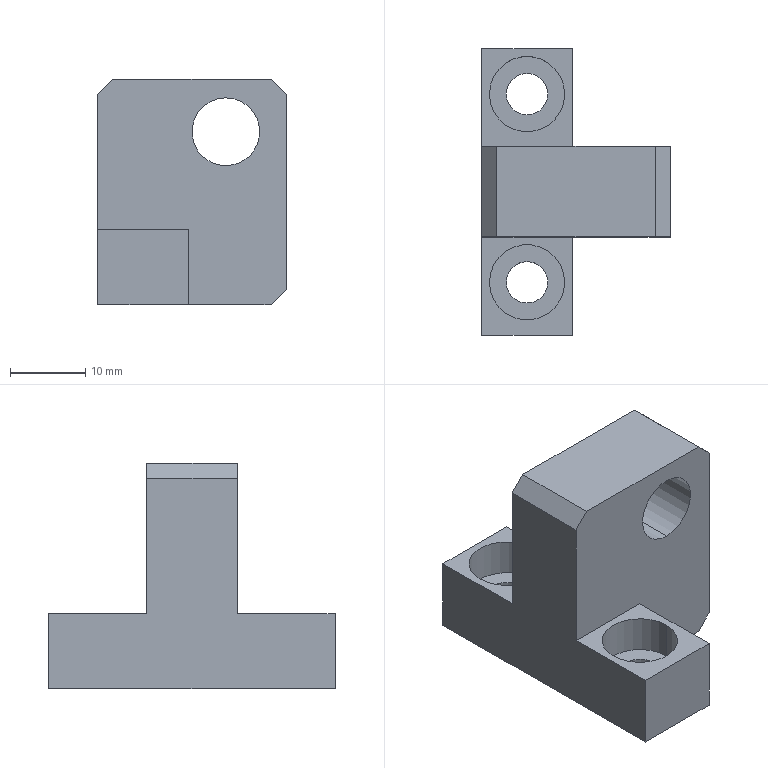Part | STEP file | 11-FG-E00311 | 1 solid | 27 faces | box 25 x 38 x 30 mm | volume 10262 mm3 | plane 17 | cylinder 10 | commonest cylinder face diameters 5.5 x4 10 x4 9 x2
STEP:
#1=CARTESIAN_POINT('',(-8.993,4.797,18.5));
#2=VERTEX_POINT('',#1);
#3=CARTESIAN_POINT('',(-8.993,4.797,27.5));
#4=VERTEX_POINT('',#3);
#5=CARTESIAN_POINT('',(-8.993,4.797,23.));
#6=DIRECTION('',(0.,1.,0.));
#7=DIRECTION('',(-1.,0.,0.));
#8=AXIS2_PLACEMENT_3D('',#5,#6,#7);
#9=CIRCLE('',#8,4.5);
#10=EDGE_CURVE('',#2,#4,#9,.T.);
#11=ORIENTED_EDGE('',*,*,#10,.F.);
#12=CARTESIAN_POINT('',(-8.993,16.797,18.5));
#13=VERTEX_POINT('',#12);
#14=CARTESIAN_POINT('',(-8.993,16.797,18.5));
#15=DIRECTION('',(0.,1.,0.));
#16=VECTOR('',#15,1000.);
#17=LINE('',#14,#16);
#18=EDGE_CURVE('',#2,#13,#17,.T.);
#19=ORIENTED_EDGE('',*,*,#18,.T.);
#20=CARTESIAN_POINT('',(-8.993,16.797,27.5));
#21=VERTEX_POINT('',#20);
#22=CARTESIAN_POINT('',(-8.993,16.797,23.));
#23=DIRECTION('',(0.,1.,0.));
#24=DIRECTION('',(0.,0.,1.));
#25=AXIS2_PLACEMENT_3D('',#22,#23,#24);
#26=CIRCLE('',#25,4.5);
#27=EDGE_CURVE('',#13,#21,#26,.T.);
#28=ORIENTED_EDGE('',*,*,#27,.T.);
#29=CARTESIAN_POINT('',(-8.993,16.797,27.5));
#30=DIRECTION('',(0.,1.,0.));
#31=VECTOR('',#30,1000.);
#32=LINE('',#29,#31);
#33=EDGE_CURVE('',#4,#21,#32,.T.);
#34=ORIENTED_EDGE('',*,*,#33,.F.);
#35=EDGE_LOOP('',(#11,#19,#28,#34));
#36=FACE_OUTER_BOUND('',#35,.T.);
#37=CARTESIAN_POINT('',(-8.993,16.797,23.));
#38=DIRECTION('',(0.,1.,0.));
#39=DIRECTION('',(0.,0.,1.));
#40=AXIS2_PLACEMENT_3D('',#37,#38,#39);
#41=CYLINDRICAL_SURFACE('',#40,4.5);
#42=ADVANCED_FACE('',(#36),#41,.F.);
#43=CARTESIAN_POINT('',(-24.993,23.797,5.));
#44=VERTEX_POINT('',#43);
#45=CARTESIAN_POINT('',(-14.993,23.797,5.));
#46=VERTEX_POINT('',#45);
#47=CARTESIAN_POINT('',(-19.993,23.797,5.));
#48=DIRECTION('',(0.,0.,1.));
#49=DIRECTION('',(1.,0.,0.));
#50=AXIS2_PLACEMENT_3D('',#47,#48,#49);
#51=CIRCLE('',#50,5.);
#52=EDGE_CURVE('',#44,#46,#51,.T.);
#53=ORIENTED_EDGE('',*,*,#52,.F.);
#54=CARTESIAN_POINT('',(-24.993,23.797,10.));
#55=VERTEX_POINT('',#54);
#56=CARTESIAN_POINT('',(-24.993,23.797,10.));
#57=DIRECTION('',(0.,0.,1.));
#58=VECTOR('',#57,1000.);
#59=LINE('',#56,#58);
#60=EDGE_CURVE('',#44,#55,#59,.T.);
#61=ORIENTED_EDGE('',*,*,#60,.T.);
#62=CARTESIAN_POINT('',(-14.993,23.797,10.));
#63=VERTEX_POINT('',#62);
#64=CARTESIAN_POINT('',(-19.993,23.797,10.));
#65=DIRECTION('',(0.,0.,1.));
#66=DIRECTION('',(1.,0.,0.));
#67=AXIS2_PLACEMENT_3D('',#64,#65,#66);
#68=CIRCLE('',#67,5.);
#69=EDGE_CURVE('',#55,#63,#68,.T.);
#70=ORIENTED_EDGE('',*,*,#69,.T.);
#71=CARTESIAN_POINT('',(-14.993,23.797,10.));
#72=DIRECTION('',(0.,0.,1.));
#73=VECTOR('',#72,1000.);
#74=LINE('',#71,#73);
#75=EDGE_CURVE('',#46,#63,#74,.T.);
#76=ORIENTED_EDGE('',*,*,#75,.F.);
#77=EDGE_LOOP('',(#53,#61,#70,#76));
#78=FACE_OUTER_BOUND('',#77,.T.);
#79=CARTESIAN_POINT('',(-19.993,23.797,10.));
#80=DIRECTION('',(0.,0.,1.));
#81=DIRECTION('',(1.,0.,0.));
#82=AXIS2_PLACEMENT_3D('',#79,#80,#81);
#83=CYLINDRICAL_SURFACE('',#82,5.);
#84=ADVANCED_FACE('',(#78),#83,.F.);
#85=CARTESIAN_POINT('',(-22.743,23.797,0.));
#86=VERTEX_POINT('',#85);
#87=CARTESIAN_POINT('',(-17.243,23.797,0.));
#88=VERTEX_POINT('',#87);
#89=CARTESIAN_POINT('',(-19.993,23.797,0.));
#90=DIRECTION('',(0.,0.,1.));
#91=DIRECTION('',(1.,0.,0.));
#92=AXIS2_PLACEMENT_3D('',#89,#90,#91);
#93=CIRCLE('',#92,2.75);
#94=EDGE_CURVE('',#86,#88,#93,.T.);
#95=ORIENTED_EDGE('',*,*,#94,.F.);
#96=CARTESIAN_POINT('',(-22.743,23.797,5.));
#97=VERTEX_POINT('',#96);
#98=CARTESIAN_POINT('',(-22.743,23.797,10.));
#99=DIRECTION('',(0.,0.,1.));
#100=VECTOR('',#99,1000.);
#101=LINE('',#98,#100);
#102=EDGE_CURVE('',#86,#97,#101,.T.);
#103=ORIENTED_EDGE('',*,*,#102,.T.);
#104=CARTESIAN_POINT('',(-17.243,23.797,5.));
#105=VERTEX_POINT('',#104);
#106=CARTESIAN_POINT('',(-19.993,23.797,5.));
#107=DIRECTION('',(0.,0.,1.));
#108=DIRECTION('',(1.,0.,0.));
#109=AXIS2_PLACEMENT_3D('',#106,#107,#108);
#110=CIRCLE('',#109,2.75);
#111=EDGE_CURVE('',#97,#105,#110,.T.);
#112=ORIENTED_EDGE('',*,*,#111,.T.);
#113=CARTESIAN_POINT('',(-17.243,23.797,10.));
#114=DIRECTION('',(0.,0.,1.));
#115=VECTOR('',#114,1000.);
#116=LINE('',#113,#115);
#117=EDGE_CURVE('',#88,#105,#116,.T.);
#118=ORIENTED_EDGE('',*,*,#117,.F.);
#119=EDGE_LOOP('',(#95,#103,#112,#118));
#120=FACE_OUTER_BOUND('',#119,.T.);
#121=CARTESIAN_POINT('',(-19.993,23.797,10.));
#122=DIRECTION('',(0.,0.,1.));
#123=DIRECTION('',(1.,0.,0.));
#124=AXIS2_PLACEMENT_3D('',#121,#122,#123);
#125=CYLINDRICAL_SURFACE('',#124,2.75);
#126=ADVANCED_FACE('',(#120),#125,.F.);
#127=CARTESIAN_POINT('',(-24.993,-1.203,5.));
#128=VERTEX_POINT('',#127);
#129=CARTESIAN_POINT('',(-14.993,-1.203,5.));
#130=VERTEX_POINT('',#129);
#131=CARTESIAN_POINT('',(-19.993,-1.203,5.));
#132=DIRECTION('',(0.,0.,1.));
#133=DIRECTION('',(1.,0.,0.));
#134=AXIS2_PLACEMENT_3D('',#131,#132,#133);
#135=CIRCLE('',#134,5.);
#136=EDGE_CURVE('',#128,#130,#135,.T.);
#137=ORIENTED_EDGE('',*,*,#136,.F.);
#138=CARTESIAN_POINT('',(-24.993,-1.203,10.));
#139=VERTEX_POINT('',#138);
#140=CARTESIAN_POINT('',(-24.993,-1.203,10.));
#141=DIRECTION('',(0.,0.,1.));
#142=VECTOR('',#141,1000.);
#143=LINE('',#140,#142);
#144=EDGE_CURVE('',#128,#139,#143,.T.);
#145=ORIENTED_EDGE('',*,*,#144,.T.);
#146=CARTESIAN_POINT('',(-14.993,-1.203,10.));
#147=VERTEX_POINT('',#146);
#148=CARTESIAN_POINT('',(-19.993,-1.203,10.));
#149=DIRECTION('',(0.,0.,1.));
#150=DIRECTION('',(1.,0.,0.));
#151=AXIS2_PLACEMENT_3D('',#148,#149,#150);
#152=CIRCLE('',#151,5.);
#153=EDGE_CURVE('',#139,#147,#152,.T.);
#154=ORIENTED_EDGE('',*,*,#153,.T.);
#155=CARTESIAN_POINT('',(-14.993,-1.203,10.));
#156=DIRECTION('',(0.,0.,1.));
#157=VECTOR('',#156,1000.);
#158=LINE('',#155,#157);
#159=EDGE_CURVE('',#130,#147,#158,.T.);
#160=ORIENTED_EDGE('',*,*,#159,.F.);
#161=EDGE_LOOP('',(#137,#145,#154,#160));
#162=FACE_OUTER_BOUND('',#161,.T.);
#163=CARTESIAN_POINT('',(-19.993,-1.203,10.));
#164=DIRECTION('',(0.,0.,1.));
#165=DIRECTION('',(1.,0.,0.));
#166=AXIS2_PLACEMENT_3D('',#163,#164,#165);
#167=CYLINDRICAL_SURFACE('',#166,5.);
#168=ADVANCED_FACE('',(#162),#167,.F.);
#169=CARTESIAN_POINT('',(-22.743,-1.203,0.));
#170=VERTEX_POINT('',#169);
#171=CARTESIAN_POINT('',(-17.243,-1.203,0.));
#172=VERTEX_POINT('',#171);
#173=CARTESIAN_POINT('',(-19.993,-1.203,0.));
#174=DIRECTION('',(0.,0.,1.));
#175=DIRECTION('',(1.,0.,0.));
#176=AXIS2_PLACEMENT_3D('',#173,#174,#175);
#177=CIRCLE('',#176,2.75);
#178=EDGE_CURVE('',#170,#172,#177,.T.);
#179=ORIENTED_EDGE('',*,*,#178,.F.);
#180=CARTESIAN_POINT('',(-22.743,-1.203,5.));
#181=VERTEX_POINT('',#180);
#182=CARTESIAN_POINT('',(-22.743,-1.203,10.));
#183=DIRECTION('',(0.,0.,1.));
#184=VECTOR('',#183,1000.);
#185=LINE('',#182,#184);
#186=EDGE_CURVE('',#170,#181,#185,.T.);
#187=ORIENTED_EDGE('',*,*,#186,.T.);
#188=CARTESIAN_POINT('',(-17.243,-1.203,5.));
#189=VERTEX_POINT('',#188);
#190=CARTESIAN_POINT('',(-19.993,-1.203,5.));
#191=DIRECTION('',(0.,0.,1.));
#192=DIRECTION('',(1.,0.,0.));
#193=AXIS2_PLACEMENT_3D('',#190,#191,#192);
#194=CIRCLE('',#193,2.75);
#195=EDGE_CURVE('',#181,#189,#194,.T.);
#196=ORIENTED_EDGE('',*,*,#195,.T.);
#197=CARTESIAN_POINT('',(-17.243,-1.203,10.));
#198=DIRECTION('',(0.,0.,1.));
#199=VECTOR('',#198,1000.);
#200=LINE('',#197,#199);
#201=EDGE_CURVE('',#172,#189,#200,.T.);
#202=ORIENTED_EDGE('',*,*,#201,.F.);
#203=EDGE_LOOP('',(#179,#187,#196,#202));
#204=FACE_OUTER_BOUND('',#203,.T.);
#205=CARTESIAN_POINT('',(-19.993,-1.203,10.));
#206=DIRECTION('',(0.,0.,1.));
#207=DIRECTION('',(1.,0.,0.));
#208=AXIS2_PLACEMENT_3D('',#205,#206,#207);
#209=CYLINDRICAL_SURFACE('',#208,2.75);
#210=ADVANCED_FACE('',(#204),#209,.F.);
#211=CARTESIAN_POINT('',(-13.993,16.797,10.));
#212=VERTEX_POINT('',#211);
#213=CARTESIAN_POINT('',(-25.993,16.797,10.));
#214=VERTEX_POINT('',#213);
#215=CARTESIAN_POINT('',(-0.9932,16.797,10.));
#216=DIRECTION('',(-1.,0.,0.));
#217=VECTOR('',#216,1000.);
#218=LINE('',#215,#217);
#219=EDGE_CURVE('',#212,#214,#218,.T.);
#220=ORIENTED_EDGE('',*,*,#219,.F.);
#221=CARTESIAN_POINT('',(-13.993,29.797,10.));
#222=VERTEX_POINT('',#221);
#223=CARTESIAN_POINT('',(-13.993,29.797,10.));
#224=DIRECTION('',(0.,-1.,0.));
#225=VECTOR('',#224,1000.);
#226=LINE('',#223,#225);
#227=EDGE_CURVE('',#222,#212,#226,.T.);
#228=ORIENTED_EDGE('',*,*,#227,.F.);
#229=CARTESIAN_POINT('',(-25.993,29.797,10.));
#230=VERTEX_POINT('',#229);
#231=CARTESIAN_POINT('',(-0.9932,29.797,10.));
#232=DIRECTION('',(-1.,0.,0.));
#233=VECTOR('',#232,1000.);
#234=LINE('',#231,#233);
#235=EDGE_CURVE('',#222,#230,#234,.T.);
#236=ORIENTED_EDGE('',*,*,#235,.T.);
#237=CARTESIAN_POINT('',(-25.993,16.797,10.));
#238=DIRECTION('',(0.,1.,0.));
#239=VECTOR('',#238,1000.);
#240=LINE('',#237,#239);
#241=EDGE_CURVE('',#214,#230,#240,.T.);
#242=ORIENTED_EDGE('',*,*,#241,.F.);
#243=EDGE_LOOP('',(#220,#228,#236,#242));
#244=FACE_OUTER_BOUND('',#243,.T.);
#245=CARTESIAN_POINT('',(-19.993,23.797,10.));
#246=DIRECTION('',(0.,0.,1.));
#247=DIRECTION('',(1.,0.,0.));
#248=AXIS2_PLACEMENT_3D('',#245,#246,#247);
#249=CIRCLE('',#248,5.);
#250=EDGE_CURVE('',#63,#55,#249,.T.);
#251=ORIENTED_EDGE('',*,*,#250,.F.);
#252=ORIENTED_EDGE('',*,*,#69,.F.);
#253=EDGE_LOOP('',(#251,#252));
#254=FACE_BOUND('',#253,.T.);
#255=CARTESIAN_POINT('',(-0.9932,16.797,10.));
#256=DIRECTION('',(0.,0.,-1.));
#257=DIRECTION('',(-1.,0.,0.));
#258=AXIS2_PLACEMENT_3D('',#255,#256,#257);
#259=PLANE('',#258);
#260=ADVANCED_FACE('',(#244,#254),#259,.F.);
#261=CARTESIAN_POINT('',(-2.993,4.797,30.));
#262=VERTEX_POINT('',#261);
#263=CARTESIAN_POINT('',(-23.993,4.797,30.));
#264=VERTEX_POINT('',#263);
#265=CARTESIAN_POINT('',(-0.9932,4.797,30.));
#266=DIRECTION('',(-1.,0.,0.));
#267=VECTOR('',#266,1000.);
#268=LINE('',#265,#267);
#269=EDGE_CURVE('',#262,#264,#268,.T.);
#270=ORIENTED_EDGE('',*,*,#269,.F.);
#271=CARTESIAN_POINT('',(-2.993,16.797,30.));
#272=VERTEX_POINT('',#271);
#273=CARTESIAN_POINT('',(-2.993,16.797,30.));
#274=DIRECTION('',(0.,1.,0.));
#275=VECTOR('',#274,1000.);
#276=LINE('',#273,#275);
#277=EDGE_CURVE('',#262,#272,#276,.T.);
#278=ORIENTED_EDGE('',*,*,#277,.T.);
#279=CARTESIAN_POINT('',(-23.993,16.797,30.));
#280=VERTEX_POINT('',#279);
#281=CARTESIAN_POINT('',(-0.9932,16.797,30.));
#282=DIRECTION('',(1.,0.,0.));
#283=VECTOR('',#282,1000.);
#284=LINE('',#281,#283);
#285=EDGE_CURVE('',#280,#272,#284,.T.);
#286=ORIENTED_EDGE('',*,*,#285,.F.);
#287=CARTESIAN_POINT('',(-23.993,4.797,30.));
#288=DIRECTION('',(0.,-1.,0.));
#289=VECTOR('',#288,1000.);
#290=LINE('',#287,#289);
#291=EDGE_CURVE('',#280,#264,#290,.T.);
#292=ORIENTED_EDGE('',*,*,#291,.T.);
#293=EDGE_LOOP('',(#270,#278,#286,#292));
#294=FACE_OUTER_BOUND('',#293,.T.);
#295=CARTESIAN_POINT('',(-25.993,-20.203,30.));
#296=DIRECTION('',(0.,0.,1.));
#297=DIRECTION('',(1.,0.,0.));
#298=AXIS2_PLACEMENT_3D('',#295,#296,#297);
#299=PLANE('',#298);
#300=ADVANCED_FACE('',(#294),#299,.T.);
#301=CARTESIAN_POINT('',(-25.993,4.797,10.));
#302=VERTEX_POINT('',#301);
#303=CARTESIAN_POINT('',(-25.993,4.797,28.));
#304=VERTEX_POINT('',#303);
#305=CARTESIAN_POINT('',(-25.993,4.797,10.));
#306=DIRECTION('',(0.,0.,1.));
#307=VECTOR('',#306,1000.);
#308=LINE('',#305,#307);
#309=EDGE_CURVE('',#302,#304,#308,.T.);
#310=ORIENTED_EDGE('',*,*,#309,.T.);
#311=CARTESIAN_POINT('',(-25.993,16.797,28.));
#312=VERTEX_POINT('',#311);
#313=CARTESIAN_POINT('',(-25.993,16.797,28.));
#314=DIRECTION('',(0.,1.,0.));
#315=VECTOR('',#314,1000.);
#316=LINE('',#313,#315);
#317=EDGE_CURVE('',#304,#312,#316,.T.);
#318=ORIENTED_EDGE('',*,*,#317,.T.);
#319=CARTESIAN_POINT('',(-25.993,16.797,30.));
#320=DIRECTION('',(0.,0.,1.));
#321=VECTOR('',#320,1000.);
#322=LINE('',#319,#321);
#323=EDGE_CURVE('',#214,#312,#322,.T.);
#324=ORIENTED_EDGE('',*,*,#323,.F.);
#325=ORIENTED_EDGE('',*,*,#241,.T.);
#326=CARTESIAN_POINT('',(-25.993,29.797,0.));
#327=VERTEX_POINT('',#326);
#328=CARTESIAN_POINT('',(-25.993,29.797,30.));
#329=DIRECTION('',(0.,0.,-1.));
#330=VECTOR('',#329,1000.);
#331=LINE('',#328,#330);
#332=EDGE_CURVE('',#230,#327,#331,.T.);
#333=ORIENTED_EDGE('',*,*,#332,.T.);
#334=CARTESIAN_POINT('',(-25.993,-8.203,0.));
#335=VERTEX_POINT('',#334);
#336=CARTESIAN_POINT('',(-25.993,29.797,0.));
#337=DIRECTION('',(0.,-1.,0.));
#338=VECTOR('',#337,1000.);
#339=LINE('',#336,#338);
#340=EDGE_CURVE('',#327,#335,#339,.T.);
#341=ORIENTED_EDGE('',*,*,#340,.T.);
#342=CARTESIAN_POINT('',(-25.993,-8.203,10.));
#343=VERTEX_POINT('',#342);
#344=CARTESIAN_POINT('',(-25.993,-8.203,0.));
#345=DIRECTION('',(0.,0.,1.));
#346=VECTOR('',#345,1000.);
#347=LINE('',#344,#346);
#348=EDGE_CURVE('',#335,#343,#347,.T.);
#349=ORIENTED_EDGE('',*,*,#348,.T.);
#350=CARTESIAN_POINT('',(-25.993,-20.203,10.));
#351=DIRECTION('',(0.,-1.,0.));
#352=VECTOR('',#351,1000.);
#353=LINE('',#350,#352);
#354=EDGE_CURVE('',#302,#343,#353,.T.);
#355=ORIENTED_EDGE('',*,*,#354,.F.);
#356=EDGE_LOOP('',(#310,#318,#324,#325,#333,#341,#349,#355));
#357=FACE_OUTER_BOUND('',#356,.T.);
#358=CARTESIAN_POINT('',(-25.993,29.797,30.));
#359=DIRECTION('',(1.,0.,0.));
#360=DIRECTION('',(0.,1.,0.));
#361=AXIS2_PLACEMENT_3D('',#358,#359,#360);
#362=PLANE('',#361);
#363=ADVANCED_FACE('',(#357),#362,.F.);
#364=CARTESIAN_POINT('',(-0.9932,4.797,2.));
#365=VERTEX_POINT('',#364);
#366=CARTESIAN_POINT('',(-0.9932,4.797,28.));
#367=VERTEX_POINT('',#366);
#368=CARTESIAN_POINT('',(-0.9932,4.797,10.));
#369=DIRECTION('',(0.,0.,1.));
#370=VECTOR('',#369,1000.);
#371=LINE('',#368,#370);
#372=EDGE_CURVE('',#365,#367,#371,.T.);
#373=ORIENTED_EDGE('',*,*,#372,.F.);
#374=CARTESIAN_POINT('',(-0.9932,16.797,2.));
#375=VERTEX_POINT('',#374);
#376=CARTESIAN_POINT('',(-0.9932,29.797,2.));
#377=DIRECTION('',(0.,1.,0.));
#378=VECTOR('',#377,1000.);
#379=LINE('',#376,#378);
#380=EDGE_CURVE('',#365,#375,#379,.T.);
#381=ORIENTED_EDGE('',*,*,#380,.T.);
#382=CARTESIAN_POINT('',(-0.9932,16.797,28.));
#383=VERTEX_POINT('',#382);
#384=CARTESIAN_POINT('',(-0.9932,16.797,30.));
#385=DIRECTION('',(0.,0.,-1.));
#386=VECTOR('',#385,1000.);
#387=LINE('',#384,#386);
#388=EDGE_CURVE('',#383,#375,#387,.T.);
#389=ORIENTED_EDGE('',*,*,#388,.F.);
#390=CARTESIAN_POINT('',(-0.9932,4.797,28.));
#391=DIRECTION('',(0.,-1.,0.));
#392=VECTOR('',#391,1000.);
#393=LINE('',#390,#392);
#394=EDGE_CURVE('',#383,#367,#393,.T.);
#395=ORIENTED_EDGE('',*,*,#394,.T.);
#396=EDGE_LOOP('',(#373,#381,#389,#395));
#397=FACE_OUTER_BOUND('',#396,.T.);
#398=CARTESIAN_POINT('',(-0.9932,29.797,30.));
#399=DIRECTION('',(-1.,0.,0.));
#400=DIRECTION('',(0.,-1.,0.));
#401=AXIS2_PLACEMENT_3D('',#398,#399,#400);
#402=PLANE('',#401);
#403=ADVANCED_FACE('',(#397),#402,.F.);
#404=ORIENTED_EDGE('',*,*,#235,.F.);
#405=CARTESIAN_POINT('',(-13.993,29.797,0.));
#406=VERTEX_POINT('',#405);
#407=CARTESIAN_POINT('',(-13.993,29.797,0.));
#408=DIRECTION('',(0.,0.,1.));
#409=VECTOR('',#408,1000.);
#410=LINE('',#407,#409);
#411=EDGE_CURVE('',#406,#222,#410,.T.);
#412=ORIENTED_EDGE('',*,*,#411,.F.);
#413=CARTESIAN_POINT('',(-25.993,29.797,0.));
#414=DIRECTION('',(-1.,0.,0.));
#415=VECTOR('',#414,1000.);
#416=LINE('',#413,#415);
#417=EDGE_CURVE('',#406,#327,#416,.T.);
#418=ORIENTED_EDGE('',*,*,#417,.T.);
#419=ORIENTED_EDGE('',*,*,#332,.F.);
#420=EDGE_LOOP('',(#404,#412,#418,#419));
#421=FACE_OUTER_BOUND('',#420,.T.);
#422=CARTESIAN_POINT('',(-25.993,29.797,30.));
#423=DIRECTION('',(0.,-1.,0.));
#424=DIRECTION('',(0.,0.,-1.));
#425=AXIS2_PLACEMENT_3D('',#422,#423,#424);
#426=PLANE('',#425);
#427=ADVANCED_FACE('',(#421),#426,.F.);
#428=CARTESIAN_POINT('',(-19.993,23.797,0.));
#429=DIRECTION('',(0.,0.,1.));
#430=DIRECTION('',(1.,0.,0.));
#431=AXIS2_PLACEMENT_3D('',#428,#429,#430);
#432=CIRCLE('',#431,2.75);
#433=EDGE_CURVE('',#88,#86,#432,.T.);
#434=ORIENTED_EDGE('',*,*,#433,.T.);
#435=ORIENTED_EDGE('',*,*,#94,.T.);
#436=EDGE_LOOP('',(#434,#435));
#437=FACE_BOUND('',#436,.T.);
#438=CARTESIAN_POINT('',(-19.993,-1.203,0.));
#439=DIRECTION('',(0.,0.,1.));
#440=DIRECTION('',(1.,0.,0.));
#441=AXIS2_PLACEMENT_3D('',#438,#439,#440);
#442=CIRCLE('',#441,2.75);
#443=EDGE_CURVE('',#172,#170,#442,.T.);
#444=ORIENTED_EDGE('',*,*,#443,.T.);
#445=ORIENTED_EDGE('',*,*,#178,.T.);
#446=EDGE_LOOP('',(#444,#445));
#447=FACE_BOUND('',#446,.T.);
#448=CARTESIAN_POINT('',(-13.993,16.797,0.));
#449=VERTEX_POINT('',#448);
#450=CARTESIAN_POINT('',(-2.993,16.797,0.));
#451=VERTEX_POINT('',#450);
#452=CARTESIAN_POINT('',(-0.9932,16.797,0.));
#453=DIRECTION('',(1.,0.,0.));
#454=VECTOR('',#453,1000.);
#455=LINE('',#452,#454);
#456=EDGE_CURVE('',#449,#451,#455,.T.);
#457=ORIENTED_EDGE('',*,*,#456,.T.);
#458=CARTESIAN_POINT('',(-2.993,4.797,0.));
#459=VERTEX_POINT('',#458);
#460=CARTESIAN_POINT('',(-2.993,-20.203,0.));
#461=DIRECTION('',(0.,-1.,0.));
#462=VECTOR('',#461,1000.);
#463=LINE('',#460,#462);
#464=EDGE_CURVE('',#451,#459,#463,.T.);
#465=ORIENTED_EDGE('',*,*,#464,.T.);
#466=CARTESIAN_POINT('',(-13.993,4.797,0.));
#467=VERTEX_POINT('',#466);
#468=CARTESIAN_POINT('',(-0.9932,4.797,0.));
#469=DIRECTION('',(-1.,0.,0.));
#470=VECTOR('',#469,1000.);
#471=LINE('',#468,#470);
#472=EDGE_CURVE('',#459,#467,#471,.T.);
#473=ORIENTED_EDGE('',*,*,#472,.T.);
#474=CARTESIAN_POINT('',(-13.993,-8.203,0.));
#475=VERTEX_POINT('',#474);
#476=CARTESIAN_POINT('',(-13.993,-20.203,0.));
#477=DIRECTION('',(0.,-1.,0.));
#478=VECTOR('',#477,1000.);
#479=LINE('',#476,#478);
#480=EDGE_CURVE('',#467,#475,#479,.T.);
#481=ORIENTED_EDGE('',*,*,#480,.T.);
#482=CARTESIAN_POINT('',(-25.993,-8.203,0.));
#483=DIRECTION('',(-1.,0.,0.));
#484=VECTOR('',#483,1000.);
#485=LINE('',#482,#484);
#486=EDGE_CURVE('',#475,#335,#485,.T.);
#487=ORIENTED_EDGE('',*,*,#486,.T.);
#488=ORIENTED_EDGE('',*,*,#340,.F.);
#489=ORIENTED_EDGE('',*,*,#417,.F.);
#490=CARTESIAN_POINT('',(-13.993,29.797,0.));
#491=DIRECTION('',(0.,-1.,0.));
#492=VECTOR('',#491,1000.);
#493=LINE('',#490,#492);
#494=EDGE_CURVE('',#406,#449,#493,.T.);
#495=ORIENTED_EDGE('',*,*,#494,.T.);
#496=EDGE_LOOP('',(#457,#465,#473,#481,#487,#488,#489,#495));
#497=FACE_OUTER_BOUND('',#496,.T.);
#498=CARTESIAN_POINT('',(-25.993,-20.203,0.));
#499=DIRECTION('',(0.,0.,1.));
#500=DIRECTION('',(1.,0.,0.));
#501=AXIS2_PLACEMENT_3D('',#498,#499,#500);
#502=PLANE('',#501);
#503=ADVANCED_FACE('',(#437,#447,#497),#502,.F.);
#504=CARTESIAN_POINT('',(-8.993,16.797,23.));
#505=DIRECTION('',(0.,1.,0.));
#506=DIRECTION('',(0.,0.,1.));
#507=AXIS2_PLACEMENT_3D('',#504,#505,#506);
#508=CIRCLE('',#507,4.5);
#509=EDGE_CURVE('',#21,#13,#508,.T.);
#510=ORIENTED_EDGE('',*,*,#509,.F.);
#511=ORIENTED_EDGE('',*,*,#27,.F.);
#512=EDGE_LOOP('',(#510,#511));
#513=FACE_BOUND('',#512,.T.);
#514=ORIENTED_EDGE('',*,*,#388,.T.);
#515=CARTESIAN_POINT('',(3.007,16.797,6.));
#516=DIRECTION('',(-0.7071,0.,-0.7071));
#517=VECTOR('',#516,1000.);
#518=LINE('',#515,#517);
#519=EDGE_CURVE('',#375,#451,#518,.T.);
#520=ORIENTED_EDGE('',*,*,#519,.T.);
#521=ORIENTED_EDGE('',*,*,#456,.F.);
#522=CARTESIAN_POINT('',(-13.993,16.797,0.));
#523=DIRECTION('',(0.,0.,1.));
#524=VECTOR('',#523,1000.);
#525=LINE('',#522,#524);
#526=EDGE_CURVE('',#449,#212,#525,.T.);
#527=ORIENTED_EDGE('',*,*,#526,.T.);
#528=ORIENTED_EDGE('',*,*,#219,.T.);
#529=ORIENTED_EDGE('',*,*,#323,.T.);
#530=CARTESIAN_POINT('',(-22.493,16.797,31.5));
#531=DIRECTION('',(0.7071,0.,0.7071));
#532=VECTOR('',#531,1000.);
#533=LINE('',#530,#532);
#534=EDGE_CURVE('',#312,#280,#533,.T.);
#535=ORIENTED_EDGE('',*,*,#534,.T.);
#536=ORIENTED_EDGE('',*,*,#285,.T.);
#537=CARTESIAN_POINT('',(8.007,16.797,19.));
#538=DIRECTION('',(0.7071,0.,-0.7071));
#539=VECTOR('',#538,1000.);
#540=LINE('',#537,#539);
#541=EDGE_CURVE('',#272,#383,#540,.T.);
#542=ORIENTED_EDGE('',*,*,#541,.T.);
#543=EDGE_LOOP('',(#514,#520,#521,#527,#528,#529,#535,#536,#542));
#544=FACE_OUTER_BOUND('',#543,.T.);
#545=CARTESIAN_POINT('',(-0.9932,16.797,10.));
#546=DIRECTION('',(0.,1.,0.));
#547=DIRECTION('',(0.,0.,1.));
#548=AXIS2_PLACEMENT_3D('',#545,#546,#547);
#549=PLANE('',#548);
#550=ADVANCED_FACE('',(#513,#544),#549,.T.);
#551=ORIENTED_EDGE('',*,*,#227,.T.);
#552=ORIENTED_EDGE('',*,*,#526,.F.);
#553=ORIENTED_EDGE('',*,*,#494,.F.);
#554=ORIENTED_EDGE('',*,*,#411,.T.);
#555=EDGE_LOOP('',(#551,#552,#553,#554));
#556=FACE_OUTER_BOUND('',#555,.T.);
#557=CARTESIAN_POINT('',(-13.993,29.797,0.));
#558=DIRECTION('',(-1.,0.,0.));
#559=DIRECTION('',(0.,-1.,0.));
#560=AXIS2_PLACEMENT_3D('',#557,#558,#559);
#561=PLANE('',#560);
#562=ADVANCED_FACE('',(#556),#561,.F.);
#563=ORIENTED_EDGE('',*,*,#472,.F.);
#564=CARTESIAN_POINT('',(-0.9932,4.797,2.));
#565=DIRECTION('',(0.7071,0.,0.7071));
#566=VECTOR('',#565,1000.);
#567=LINE('',#564,#566);
#568=EDGE_CURVE('',#459,#365,#567,.T.);
#569=ORIENTED_EDGE('',*,*,#568,.T.);
#570=ORIENTED_EDGE('',*,*,#372,.T.);
#571=CARTESIAN_POINT('',(-2.993,4.797,30.));
#572=DIRECTION('',(-0.7071,0.,0.7071));
#573=VECTOR('',#572,1000.);
#574=LINE('',#571,#573);
#575=EDGE_CURVE('',#367,#262,#574,.T.);
#576=ORIENTED_EDGE('',*,*,#575,.T.);
#577=ORIENTED_EDGE('',*,*,#269,.T.);
#578=CARTESIAN_POINT('',(-23.993,4.797,30.));
#579=DIRECTION('',(-0.7071,0.,-0.7071));
#580=VECTOR('',#579,1000.);
#581=LINE('',#578,#580);
#582=EDGE_CURVE('',#264,#304,#581,.T.);
#583=ORIENTED_EDGE('',*,*,#582,.T.);
#584=ORIENTED_EDGE('',*,*,#309,.F.);
#585=CARTESIAN_POINT('',(-13.993,4.797,10.));
#586=VERTEX_POINT('',#585);
#587=CARTESIAN_POINT('',(-0.9932,4.797,10.));
#588=DIRECTION('',(-1.,0.,0.));
#589=VECTOR('',#588,1000.);
#590=LINE('',#587,#589);
#591=EDGE_CURVE('',#586,#302,#590,.T.);
#592=ORIENTED_EDGE('',*,*,#591,.F.);
#593=CARTESIAN_POINT('',(-13.993,4.797,0.));
#594=DIRECTION('',(0.,0.,1.));
#595=VECTOR('',#594,1000.);
#596=LINE('',#593,#595);
#597=EDGE_CURVE('',#467,#586,#596,.T.);
#598=ORIENTED_EDGE('',*,*,#597,.F.);
#599=EDGE_LOOP('',(#563,#569,#570,#576,#577,#583,#584,#592,#598));
#600=FACE_OUTER_BOUND('',#599,.T.);
#601=CARTESIAN_POINT('',(-8.993,4.797,23.));
#602=DIRECTION('',(0.,1.,0.));
#603=DIRECTION('',(-1.,0.,0.));
#604=AXIS2_PLACEMENT_3D('',#601,#602,#603);
#605=CIRCLE('',#604,4.5);
#606=EDGE_CURVE('',#4,#2,#605,.T.);
#607=ORIENTED_EDGE('',*,*,#606,.T.);
#608=ORIENTED_EDGE('',*,*,#10,.T.);
#609=EDGE_LOOP('',(#607,#608));
#610=FACE_BOUND('',#609,.T.);
#611=CARTESIAN_POINT('',(-0.9932,4.797,10.));
#612=DIRECTION('',(0.,1.,0.));
#613=DIRECTION('',(-1.,0.,0.));
#614=AXIS2_PLACEMENT_3D('',#611,#612,#613);
#615=PLANE('',#614);
#616=ADVANCED_FACE('',(#600,#610),#615,.F.);
#617=CARTESIAN_POINT('',(-13.993,-8.203,10.));
#618=VERTEX_POINT('',#617);
#619=CARTESIAN_POINT('',(-13.993,-20.203,10.));
#620=DIRECTION('',(0.,-1.,0.));
#621=VECTOR('',#620,1000.);
#622=LINE('',#619,#621);
#623=EDGE_CURVE('',#586,#618,#622,.T.);
#624=ORIENTED_EDGE('',*,*,#623,.F.);
#625=ORIENTED_EDGE('',*,*,#591,.T.);
#626=ORIENTED_EDGE('',*,*,#354,.T.);
#627=CARTESIAN_POINT('',(-25.993,-8.203,10.));
#628=DIRECTION('',(-1.,0.,0.));
#629=VECTOR('',#628,1000.);
#630=LINE('',#627,#629);
#631=EDGE_CURVE('',#618,#343,#630,.T.);
#632=ORIENTED_EDGE('',*,*,#631,.F.);
#633=EDGE_LOOP('',(#624,#625,#626,#632));
#634=FACE_OUTER_BOUND('',#633,.T.);
#635=CARTESIAN_POINT('',(-19.993,-1.203,10.));
#636=DIRECTION('',(0.,0.,1.));
#637=DIRECTION('',(1.,0.,0.));
#638=AXIS2_PLACEMENT_3D('',#635,#636,#637);
#639=CIRCLE('',#638,5.);
#640=EDGE_CURVE('',#147,#139,#639,.T.);
#641=ORIENTED_EDGE('',*,*,#640,.F.);
#642=ORIENTED_EDGE('',*,*,#153,.F.);
#643=EDGE_LOOP('',(#641,#642));
#644=FACE_BOUND('',#643,.T.);
#645=CARTESIAN_POINT('',(-0.9932,4.797,10.));
#646=DIRECTION('',(0.,0.,1.));
#647=DIRECTION('',(1.,0.,0.));
#648=AXIS2_PLACEMENT_3D('',#645,#646,#647);
#649=PLANE('',#648);
#650=ADVANCED_FACE('',(#634,#644),#649,.T.);
#651=ORIENTED_EDGE('',*,*,#486,.F.);
#652=CARTESIAN_POINT('',(-13.993,-8.203,0.));
#653=DIRECTION('',(0.,0.,1.));
#654=VECTOR('',#653,1000.);
#655=LINE('',#652,#654);
#656=EDGE_CURVE('',#475,#618,#655,.T.);
#657=ORIENTED_EDGE('',*,*,#656,.T.);
#658=ORIENTED_EDGE('',*,*,#631,.T.);
#659=ORIENTED_EDGE('',*,*,#348,.F.);
#660=EDGE_LOOP('',(#651,#657,#658,#659));
#661=FACE_OUTER_BOUND('',#660,.T.);
#662=CARTESIAN_POINT('',(-25.993,-8.203,0.));
#663=DIRECTION('',(0.,1.,0.));
#664=DIRECTION('',(0.,0.,1.));
#665=AXIS2_PLACEMENT_3D('',#662,#663,#664);
#666=PLANE('',#665);
#667=ADVANCED_FACE('',(#661),#666,.F.);
#668=ORIENTED_EDGE('',*,*,#186,.F.);
#669=ORIENTED_EDGE('',*,*,#443,.F.);
#670=ORIENTED_EDGE('',*,*,#201,.T.);
#671=CARTESIAN_POINT('',(-19.993,-1.203,5.));
#672=DIRECTION('',(0.,0.,1.));
#673=DIRECTION('',(1.,0.,0.));
#674=AXIS2_PLACEMENT_3D('',#671,#672,#673);
#675=CIRCLE('',#674,2.75);
#676=EDGE_CURVE('',#189,#181,#675,.T.);
#677=ORIENTED_EDGE('',*,*,#676,.T.);
#678=EDGE_LOOP('',(#668,#669,#670,#677));
#679=FACE_OUTER_BOUND('',#678,.T.);
#680=CARTESIAN_POINT('',(-19.993,-1.203,10.));
#681=DIRECTION('',(0.,0.,1.));
#682=DIRECTION('',(1.,0.,0.));
#683=AXIS2_PLACEMENT_3D('',#680,#681,#682);
#684=CYLINDRICAL_SURFACE('',#683,2.75);
#685=ADVANCED_FACE('',(#679),#684,.F.);
#686=ORIENTED_EDGE('',*,*,#676,.F.);
#687=ORIENTED_EDGE('',*,*,#195,.F.);
#688=EDGE_LOOP('',(#686,#687));
#689=FACE_BOUND('',#688,.T.);
#690=CARTESIAN_POINT('',(-19.993,-1.203,5.));
#691=DIRECTION('',(0.,0.,1.));
#692=DIRECTION('',(1.,0.,0.));
#693=AXIS2_PLACEMENT_3D('',#690,#691,#692);
#694=CIRCLE('',#693,5.);
#695=EDGE_CURVE('',#130,#128,#694,.T.);
#696=ORIENTED_EDGE('',*,*,#695,.T.);
#697=ORIENTED_EDGE('',*,*,#136,.T.);
#698=EDGE_LOOP('',(#696,#697));
#699=FACE_OUTER_BOUND('',#698,.T.);
#700=CARTESIAN_POINT('',(-17.243,-1.203,5.));
#701=DIRECTION('',(0.,0.,-1.));
#702=DIRECTION('',(-1.,0.,0.));
#703=AXIS2_PLACEMENT_3D('',#700,#701,#702);
#704=PLANE('',#703);
#705=ADVANCED_FACE('',(#689,#699),#704,.F.);
#706=ORIENTED_EDGE('',*,*,#144,.F.);
#707=ORIENTED_EDGE('',*,*,#695,.F.);
#708=ORIENTED_EDGE('',*,*,#159,.T.);
#709=ORIENTED_EDGE('',*,*,#640,.T.);
#710=EDGE_LOOP('',(#706,#707,#708,#709));
#711=FACE_OUTER_BOUND('',#710,.T.);
#712=CARTESIAN_POINT('',(-19.993,-1.203,10.));
#713=DIRECTION('',(0.,0.,1.));
#714=DIRECTION('',(1.,0.,0.));
#715=AXIS2_PLACEMENT_3D('',#712,#713,#714);
#716=CYLINDRICAL_SURFACE('',#715,5.);
#717=ADVANCED_FACE('',(#711),#716,.F.);
#718=ORIENTED_EDGE('',*,*,#102,.F.);
#719=ORIENTED_EDGE('',*,*,#433,.F.);
#720=ORIENTED_EDGE('',*,*,#117,.T.);
#721=CARTESIAN_POINT('',(-19.993,23.797,5.));
#722=DIRECTION('',(0.,0.,1.));
#723=DIRECTION('',(1.,0.,0.));
#724=AXIS2_PLACEMENT_3D('',#721,#722,#723);
#725=CIRCLE('',#724,2.75);
#726=EDGE_CURVE('',#105,#97,#725,.T.);
#727=ORIENTED_EDGE('',*,*,#726,.T.);
#728=EDGE_LOOP('',(#718,#719,#720,#727));
#729=FACE_OUTER_BOUND('',#728,.T.);
#730=CARTESIAN_POINT('',(-19.993,23.797,10.));
#731=DIRECTION('',(0.,0.,1.));
#732=DIRECTION('',(1.,0.,0.));
#733=AXIS2_PLACEMENT_3D('',#730,#731,#732);
#734=CYLINDRICAL_SURFACE('',#733,2.75);
#735=ADVANCED_FACE('',(#729),#734,.F.);
#736=ORIENTED_EDGE('',*,*,#726,.F.);
#737=ORIENTED_EDGE('',*,*,#111,.F.);
#738=EDGE_LOOP('',(#736,#737));
#739=FACE_BOUND('',#738,.T.);
#740=CARTESIAN_POINT('',(-19.993,23.797,5.));
#741=DIRECTION('',(0.,0.,1.));
#742=DIRECTION('',(1.,0.,0.));
#743=AXIS2_PLACEMENT_3D('',#740,#741,#742);
#744=CIRCLE('',#743,5.);
#745=EDGE_CURVE('',#46,#44,#744,.T.);
#746=ORIENTED_EDGE('',*,*,#745,.T.);
#747=ORIENTED_EDGE('',*,*,#52,.T.);
#748=EDGE_LOOP('',(#746,#747));
#749=FACE_OUTER_BOUND('',#748,.T.);
#750=CARTESIAN_POINT('',(-17.243,23.797,5.));
#751=DIRECTION('',(0.,0.,-1.));
#752=DIRECTION('',(-1.,0.,0.));
#753=AXIS2_PLACEMENT_3D('',#750,#751,#752);
#754=PLANE('',#753);
#755=ADVANCED_FACE('',(#739,#749),#754,.F.);
#756=ORIENTED_EDGE('',*,*,#60,.F.);
#757=ORIENTED_EDGE('',*,*,#745,.F.);
#758=ORIENTED_EDGE('',*,*,#75,.T.);
#759=ORIENTED_EDGE('',*,*,#250,.T.);
#760=EDGE_LOOP('',(#756,#757,#758,#759));
#761=FACE_OUTER_BOUND('',#760,.T.);
#762=CARTESIAN_POINT('',(-19.993,23.797,10.));
#763=DIRECTION('',(0.,0.,1.));
#764=DIRECTION('',(1.,0.,0.));
#765=AXIS2_PLACEMENT_3D('',#762,#763,#764);
#766=CYLINDRICAL_SURFACE('',#765,5.);
#767=ADVANCED_FACE('',(#761),#766,.F.);
#768=ORIENTED_EDGE('',*,*,#18,.F.);
#769=ORIENTED_EDGE('',*,*,#606,.F.);
#770=ORIENTED_EDGE('',*,*,#33,.T.);
#771=ORIENTED_EDGE('',*,*,#509,.T.);
#772=EDGE_LOOP('',(#768,#769,#770,#771));
#773=FACE_OUTER_BOUND('',#772,.T.);
#774=CARTESIAN_POINT('',(-8.993,16.797,23.));
#775=DIRECTION('',(0.,1.,0.));
#776=DIRECTION('',(0.,0.,1.));
#777=AXIS2_PLACEMENT_3D('',#774,#775,#776);
#778=CYLINDRICAL_SURFACE('',#777,4.5);
#779=ADVANCED_FACE('',(#773),#778,.F.);
#780=ORIENTED_EDGE('',*,*,#480,.F.);
#781=ORIENTED_EDGE('',*,*,#597,.T.);
#782=ORIENTED_EDGE('',*,*,#623,.T.);
#783=ORIENTED_EDGE('',*,*,#656,.F.);
#784=EDGE_LOOP('',(#780,#781,#782,#783));
#785=FACE_OUTER_BOUND('',#784,.T.);
#786=CARTESIAN_POINT('',(-13.993,-20.203,0.));
#787=DIRECTION('',(-1.,0.,0.));
#788=DIRECTION('',(0.,-1.,0.));
#789=AXIS2_PLACEMENT_3D('',#786,#787,#788);
#790=PLANE('',#789);
#791=ADVANCED_FACE('',(#785),#790,.F.);
#792=ORIENTED_EDGE('',*,*,#568,.F.);
#793=ORIENTED_EDGE('',*,*,#464,.F.);
#794=ORIENTED_EDGE('',*,*,#519,.F.);
#795=ORIENTED_EDGE('',*,*,#380,.F.);
#796=EDGE_LOOP('',(#792,#793,#794,#795));
#797=FACE_OUTER_BOUND('',#796,.T.);
#798=CARTESIAN_POINT('',(-0.9932,29.797,2.));
#799=DIRECTION('',(-0.7071,0.,0.7071));
#800=DIRECTION('',(0.7071,0.,0.7071));
#801=AXIS2_PLACEMENT_3D('',#798,#799,#800);
#802=PLANE('',#801);
#803=ADVANCED_FACE('',(#797),#802,.F.);
#804=ORIENTED_EDGE('',*,*,#575,.F.);
#805=ORIENTED_EDGE('',*,*,#394,.F.);
#806=ORIENTED_EDGE('',*,*,#541,.F.);
#807=ORIENTED_EDGE('',*,*,#277,.F.);
#808=EDGE_LOOP('',(#804,#805,#806,#807));
#809=FACE_OUTER_BOUND('',#808,.T.);
#810=CARTESIAN_POINT('',(-2.993,-20.203,30.));
#811=DIRECTION('',(0.7071,0.,0.7071));
#812=DIRECTION('',(0.7071,0.,-0.7071));
#813=AXIS2_PLACEMENT_3D('',#810,#811,#812);
#814=PLANE('',#813);
#815=ADVANCED_FACE('',(#809),#814,.T.);
#816=ORIENTED_EDGE('',*,*,#534,.F.);
#817=ORIENTED_EDGE('',*,*,#317,.F.);
#818=ORIENTED_EDGE('',*,*,#582,.F.);
#819=ORIENTED_EDGE('',*,*,#291,.F.);
#820=EDGE_LOOP('',(#816,#817,#818,#819));
#821=FACE_OUTER_BOUND('',#820,.T.);
#822=CARTESIAN_POINT('',(-23.993,-20.203,30.));
#823=DIRECTION('',(-0.7071,0.,0.7071));
#824=DIRECTION('',(0.7071,0.,0.7071));
#825=AXIS2_PLACEMENT_3D('',#822,#823,#824);
#826=PLANE('',#825);
#827=ADVANCED_FACE('',(#821),#826,.T.);
#828=CLOSED_SHELL('',(#42,#84,#126,#168,#210,#260,#300,#363,#403,#427,#503,#550,#562,#616,#650,#667,#685,#705,#717,#735,#755,#767,#779,#791,#803,#815,#827));
#829=MANIFOLD_SOLID_BREP('',#828);
#830=CARTESIAN_POINT('',(0.,0.,0.));
#831=DIRECTION('',(0.,0.,1.));
#832=DIRECTION('',(1.,0.,0.));
#833=AXIS2_PLACEMENT_3D('',#830,#831,#832);
#834=(LENGTH_UNIT()NAMED_UNIT(*)SI_UNIT(.MILLI.,.METRE.));
#835=UNCERTAINTY_MEASURE_WITH_UNIT(LENGTH_MEASURE(0.00001),#834,'','');
#836=(NAMED_UNIT(*)PLANE_ANGLE_UNIT()SI_UNIT($,.RADIAN.));
#837=(NAMED_UNIT(*)SI_UNIT($,.STERADIAN.)SOLID_ANGLE_UNIT());
#838=(GEOMETRIC_REPRESENTATION_CONTEXT(3)GLOBAL_UNCERTAINTY_ASSIGNED_CONTEXT((#835))GLOBAL_UNIT_ASSIGNED_CONTEXT((#834,#836,#837))REPRESENTATION_CONTEXT('',''));
#839=ADVANCED_BREP_SHAPE_REPRESENTATION('',(#829,#833),#838);